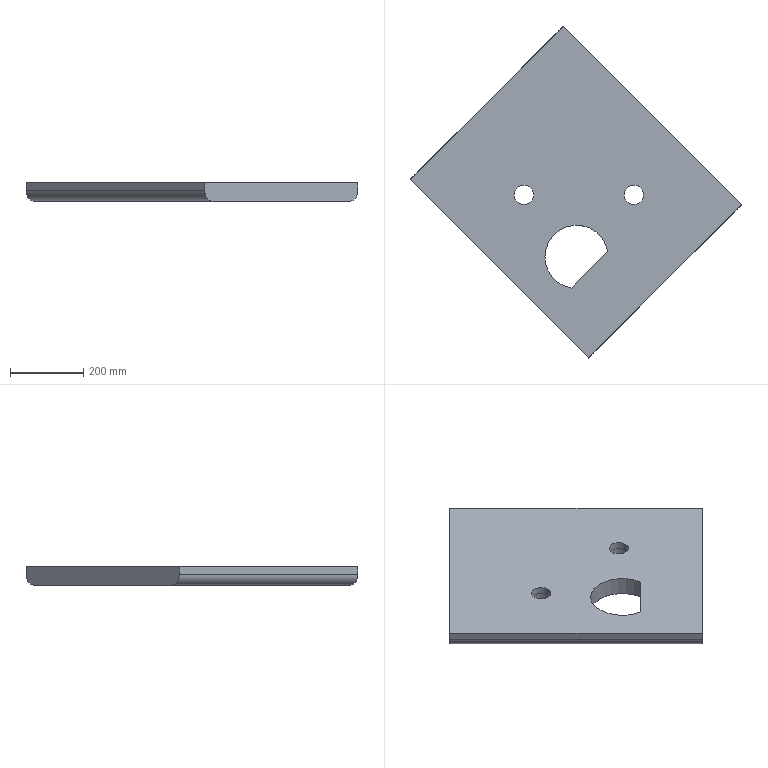Part | SolidWorks | 1 solid | 21 faces | box 906.604 x 906.604 x 50 mm | volume 18863747 mm3 | cylinder 12 | plane 9 | commonest cylinder face diameters 53 x4 68 x4 60 x2 172.729 x2
STEP:
#1=CARTESIAN_POINT('',(228.878,-154.889,-802.42));
#2=VERTEX_POINT('',#1);
#3=CARTESIAN_POINT('',(57.365,-169.327,-802.42));
#4=VERTEX_POINT('',#3);
#5=CARTESIAN_POINT('',(143.73,-169.327,-802.42));
#6=DIRECTION('',(0.,0.,1.));
#7=DIRECTION('',(0.9859,0.1672,0.));
#8=AXIS2_PLACEMENT_3D('',#5,#6,#7);
#9=CIRCLE('',#8,86.364);
#10=EDGE_CURVE('',#2,#4,#9,.T.);
#11=ORIENTED_EDGE('',*,*,#10,.T.);
#12=CARTESIAN_POINT('',(57.365,-169.327,-852.42));
#13=VERTEX_POINT('',#12);
#14=CARTESIAN_POINT('',(57.365,-169.327,-852.42));
#15=DIRECTION('',(0.,0.,-1.));
#16=VECTOR('',#15,1000.);
#17=LINE('',#14,#16);
#18=EDGE_CURVE('',#4,#13,#17,.T.);
#19=ORIENTED_EDGE('',*,*,#18,.T.);
#20=CARTESIAN_POINT('',(228.878,-154.889,-852.42));
#21=VERTEX_POINT('',#20);
#22=CARTESIAN_POINT('',(143.73,-169.327,-852.42));
#23=DIRECTION('',(0.,0.,-1.));
#24=DIRECTION('',(-0.1672,-0.9859,0.));
#25=AXIS2_PLACEMENT_3D('',#22,#23,#24);
#26=CIRCLE('',#25,86.364);
#27=EDGE_CURVE('',#13,#21,#26,.T.);
#28=ORIENTED_EDGE('',*,*,#27,.T.);
#29=CARTESIAN_POINT('',(228.878,-154.889,-802.42));
#30=DIRECTION('',(0.,0.,-1.));
#31=VECTOR('',#30,1000.);
#32=LINE('',#29,#31);
#33=EDGE_CURVE('',#2,#21,#32,.T.);
#34=ORIENTED_EDGE('',*,*,#33,.F.);
#35=EDGE_LOOP('',(#11,#19,#28,#34));
#36=FACE_OUTER_BOUND('',#35,.T.);
#37=CARTESIAN_POINT('',(143.73,-169.327,-852.42));
#38=DIRECTION('',(0.,0.,-1.));
#39=DIRECTION('',(-1.,0.,0.));
#40=AXIS2_PLACEMENT_3D('',#37,#38,#39);
#41=CYLINDRICAL_SURFACE('',#40,86.364);
#42=ADVANCED_FACE('',(#36),#41,.F.);
#43=ORIENTED_EDGE('',*,*,#18,.F.);
#44=CARTESIAN_POINT('',(129.291,-254.476,-802.42));
#45=VERTEX_POINT('',#44);
#46=CARTESIAN_POINT('',(143.73,-169.327,-802.42));
#47=DIRECTION('',(0.,0.,1.));
#48=DIRECTION('',(0.9859,0.1672,0.));
#49=AXIS2_PLACEMENT_3D('',#46,#47,#48);
#50=CIRCLE('',#49,86.364);
#51=EDGE_CURVE('',#4,#45,#50,.T.);
#52=ORIENTED_EDGE('',*,*,#51,.T.);
#53=CARTESIAN_POINT('',(129.291,-254.476,-852.42));
#54=VERTEX_POINT('',#53);
#55=CARTESIAN_POINT('',(129.291,-254.476,-852.42));
#56=DIRECTION('',(0.,0.,1.));
#57=VECTOR('',#56,1000.);
#58=LINE('',#55,#57);
#59=EDGE_CURVE('',#54,#45,#58,.T.);
#60=ORIENTED_EDGE('',*,*,#59,.F.);
#61=CARTESIAN_POINT('',(143.73,-169.327,-852.42));
#62=DIRECTION('',(0.,0.,-1.));
#63=DIRECTION('',(-0.1672,-0.9859,0.));
#64=AXIS2_PLACEMENT_3D('',#61,#62,#63);
#65=CIRCLE('',#64,86.364);
#66=EDGE_CURVE('',#54,#13,#65,.T.);
#67=ORIENTED_EDGE('',*,*,#66,.T.);
#68=EDGE_LOOP('',(#43,#52,#60,#67));
#69=FACE_OUTER_BOUND('',#68,.T.);
#70=CARTESIAN_POINT('',(143.73,-169.327,-852.42));
#71=DIRECTION('',(0.,0.,-1.));
#72=DIRECTION('',(-1.,0.,0.));
#73=AXIS2_PLACEMENT_3D('',#70,#71,#72);
#74=CYLINDRICAL_SURFACE('',#73,86.364);
#75=ADVANCED_FACE('',(#69),#74,.F.);
#76=CARTESIAN_POINT('',(129.291,-254.476,-802.42));
#77=DIRECTION('',(0.7071,0.7071,0.));
#78=VECTOR('',#77,1000.);
#79=LINE('',#76,#78);
#80=EDGE_CURVE('',#45,#2,#79,.T.);
#81=ORIENTED_EDGE('',*,*,#80,.T.);
#82=ORIENTED_EDGE('',*,*,#33,.T.);
#83=CARTESIAN_POINT('',(228.878,-154.889,-852.42));
#84=DIRECTION('',(-0.7071,-0.7071,0.));
#85=VECTOR('',#84,1000.);
#86=LINE('',#83,#85);
#87=EDGE_CURVE('',#21,#54,#86,.T.);
#88=ORIENTED_EDGE('',*,*,#87,.T.);
#89=ORIENTED_EDGE('',*,*,#59,.T.);
#90=EDGE_LOOP('',(#81,#82,#88,#89));
#91=FACE_OUTER_BOUND('',#90,.T.);
#92=CARTESIAN_POINT('',(240.322,-143.445,-852.42));
#93=DIRECTION('',(0.7071,-0.7071,0.));
#94=DIRECTION('',(0.,0.,-1.));
#95=AXIS2_PLACEMENT_3D('',#92,#93,#94);
#96=PLANE('',#95);
#97=ADVANCED_FACE('',(#91),#96,.F.);
#98=CARTESIAN_POINT('',(334.,0.,-822.42));
#99=VERTEX_POINT('',#98);
#100=CARTESIAN_POINT('',(266.,0.,-822.42));
#101=VERTEX_POINT('',#100);
#102=CARTESIAN_POINT('',(300.,0.,-822.42));
#103=DIRECTION('',(0.,0.,1.));
#104=DIRECTION('',(1.,0.,0.));
#105=AXIS2_PLACEMENT_3D('',#102,#103,#104);
#106=CIRCLE('',#105,34.);
#107=EDGE_CURVE('',#99,#101,#106,.T.);
#108=ORIENTED_EDGE('',*,*,#107,.T.);
#109=CARTESIAN_POINT('',(266.,0.,-852.42));
#110=VERTEX_POINT('',#109);
#111=CARTESIAN_POINT('',(266.,0.,-822.42));
#112=DIRECTION('',(0.,0.,-1.));
#113=VECTOR('',#112,1000.);
#114=LINE('',#111,#113);
#115=EDGE_CURVE('',#101,#110,#114,.T.);
#116=ORIENTED_EDGE('',*,*,#115,.T.);
#117=CARTESIAN_POINT('',(334.,0.,-852.42));
#118=VERTEX_POINT('',#117);
#119=CARTESIAN_POINT('',(300.,0.,-852.42));
#120=DIRECTION('',(0.,0.,-1.));
#121=DIRECTION('',(-1.,0.,0.));
#122=AXIS2_PLACEMENT_3D('',#119,#120,#121);
#123=CIRCLE('',#122,34.);
#124=EDGE_CURVE('',#110,#118,#123,.T.);
#125=ORIENTED_EDGE('',*,*,#124,.T.);
#126=CARTESIAN_POINT('',(334.,0.,-822.42));
#127=DIRECTION('',(0.,0.,-1.));
#128=VECTOR('',#127,1000.);
#129=LINE('',#126,#128);
#130=EDGE_CURVE('',#99,#118,#129,.T.);
#131=ORIENTED_EDGE('',*,*,#130,.F.);
#132=EDGE_LOOP('',(#108,#116,#125,#131));
#133=FACE_OUTER_BOUND('',#132,.T.);
#134=CARTESIAN_POINT('',(300.,0.,-852.42));
#135=DIRECTION('',(0.,0.,-1.));
#136=DIRECTION('',(-1.,0.,0.));
#137=AXIS2_PLACEMENT_3D('',#134,#135,#136);
#138=CYLINDRICAL_SURFACE('',#137,34.);
#139=ADVANCED_FACE('',(#133),#138,.F.);
#140=CARTESIAN_POINT('',(300.,0.,-822.42));
#141=DIRECTION('',(0.,0.,1.));
#142=DIRECTION('',(-1.,0.,0.));
#143=AXIS2_PLACEMENT_3D('',#140,#141,#142);
#144=CIRCLE('',#143,34.);
#145=EDGE_CURVE('',#101,#99,#144,.T.);
#146=ORIENTED_EDGE('',*,*,#145,.T.);
#147=ORIENTED_EDGE('',*,*,#130,.T.);
#148=CARTESIAN_POINT('',(300.,0.,-852.42));
#149=DIRECTION('',(0.,0.,-1.));
#150=DIRECTION('',(1.,0.,0.));
#151=AXIS2_PLACEMENT_3D('',#148,#149,#150);
#152=CIRCLE('',#151,34.);
#153=EDGE_CURVE('',#118,#110,#152,.T.);
#154=ORIENTED_EDGE('',*,*,#153,.T.);
#155=ORIENTED_EDGE('',*,*,#115,.F.);
#156=EDGE_LOOP('',(#146,#147,#154,#155));
#157=FACE_OUTER_BOUND('',#156,.T.);
#158=CARTESIAN_POINT('',(300.,0.,-852.42));
#159=DIRECTION('',(0.,0.,-1.));
#160=DIRECTION('',(-1.,0.,0.));
#161=AXIS2_PLACEMENT_3D('',#158,#159,#160);
#162=CYLINDRICAL_SURFACE('',#161,34.);
#163=ADVANCED_FACE('',(#157),#162,.F.);
#164=CARTESIAN_POINT('',(273.5,0.,-822.42));
#165=VERTEX_POINT('',#164);
#166=CARTESIAN_POINT('',(326.5,0.,-822.42));
#167=VERTEX_POINT('',#166);
#168=CARTESIAN_POINT('',(300.,0.,-822.42));
#169=DIRECTION('',(0.,0.,-1.));
#170=DIRECTION('',(-1.,0.,0.));
#171=AXIS2_PLACEMENT_3D('',#168,#169,#170);
#172=CIRCLE('',#171,26.5);
#173=EDGE_CURVE('',#165,#167,#172,.T.);
#174=ORIENTED_EDGE('',*,*,#173,.F.);
#175=CARTESIAN_POINT('',(300.,0.,-822.42));
#176=DIRECTION('',(0.,0.,-1.));
#177=DIRECTION('',(1.,0.,0.));
#178=AXIS2_PLACEMENT_3D('',#175,#176,#177);
#179=CIRCLE('',#178,26.5);
#180=EDGE_CURVE('',#167,#165,#179,.T.);
#181=ORIENTED_EDGE('',*,*,#180,.F.);
#182=EDGE_LOOP('',(#174,#181));
#183=FACE_BOUND('',#182,.T.);
#184=ORIENTED_EDGE('',*,*,#107,.F.);
#185=ORIENTED_EDGE('',*,*,#145,.F.);
#186=EDGE_LOOP('',(#184,#185));
#187=FACE_OUTER_BOUND('',#186,.T.);
#188=CARTESIAN_POINT('',(0.,0.,-822.42));
#189=DIRECTION('',(0.,0.,-1.));
#190=DIRECTION('',(0.,-1.,0.));
#191=AXIS2_PLACEMENT_3D('',#188,#189,#190);
#192=PLANE('',#191);
#193=ADVANCED_FACE('',(#183,#187),#192,.T.);
#194=CARTESIAN_POINT('',(326.5,0.,-802.42));
#195=VERTEX_POINT('',#194);
#196=CARTESIAN_POINT('',(273.5,0.,-802.42));
#197=VERTEX_POINT('',#196);
#198=CARTESIAN_POINT('',(300.,0.,-802.42));
#199=DIRECTION('',(0.,0.,1.));
#200=DIRECTION('',(1.,0.,0.));
#201=AXIS2_PLACEMENT_3D('',#198,#199,#200);
#202=CIRCLE('',#201,26.5);
#203=EDGE_CURVE('',#195,#197,#202,.T.);
#204=ORIENTED_EDGE('',*,*,#203,.T.);
#205=CARTESIAN_POINT('',(273.5,0.,-802.42));
#206=DIRECTION('',(0.,0.,-1.));
#207=VECTOR('',#206,1000.);
#208=LINE('',#205,#207);
#209=EDGE_CURVE('',#197,#165,#208,.T.);
#210=ORIENTED_EDGE('',*,*,#209,.T.);
#211=ORIENTED_EDGE('',*,*,#173,.T.);
#212=CARTESIAN_POINT('',(326.5,0.,-802.42));
#213=DIRECTION('',(0.,0.,-1.));
#214=VECTOR('',#213,1000.);
#215=LINE('',#212,#214);
#216=EDGE_CURVE('',#195,#167,#215,.T.);
#217=ORIENTED_EDGE('',*,*,#216,.F.);
#218=EDGE_LOOP('',(#204,#210,#211,#217));
#219=FACE_OUTER_BOUND('',#218,.T.);
#220=CARTESIAN_POINT('',(300.,0.,-852.42));
#221=DIRECTION('',(0.,0.,-1.));
#222=DIRECTION('',(-1.,0.,0.));
#223=AXIS2_PLACEMENT_3D('',#220,#221,#222);
#224=CYLINDRICAL_SURFACE('',#223,26.5);
#225=ADVANCED_FACE('',(#219),#224,.F.);
#226=CARTESIAN_POINT('',(300.,0.,-802.42));
#227=DIRECTION('',(0.,0.,1.));
#228=DIRECTION('',(-1.,0.,0.));
#229=AXIS2_PLACEMENT_3D('',#226,#227,#228);
#230=CIRCLE('',#229,26.5);
#231=EDGE_CURVE('',#197,#195,#230,.T.);
#232=ORIENTED_EDGE('',*,*,#231,.T.);
#233=ORIENTED_EDGE('',*,*,#216,.T.);
#234=ORIENTED_EDGE('',*,*,#180,.T.);
#235=ORIENTED_EDGE('',*,*,#209,.F.);
#236=EDGE_LOOP('',(#232,#233,#234,#235));
#237=FACE_OUTER_BOUND('',#236,.T.);
#238=CARTESIAN_POINT('',(300.,0.,-852.42));
#239=DIRECTION('',(0.,0.,-1.));
#240=DIRECTION('',(-1.,0.,0.));
#241=AXIS2_PLACEMENT_3D('',#238,#239,#240);
#242=CYLINDRICAL_SURFACE('',#241,26.5);
#243=ADVANCED_FACE('',(#237),#242,.F.);
#244=ORIENTED_EDGE('',*,*,#80,.F.);
#245=ORIENTED_EDGE('',*,*,#51,.F.);
#246=ORIENTED_EDGE('',*,*,#10,.F.);
#247=EDGE_LOOP('',(#244,#245,#246));
#248=FACE_BOUND('',#247,.T.);
#249=CARTESIAN_POINT('',(26.5,0.,-802.42));
#250=VERTEX_POINT('',#249);
#251=CARTESIAN_POINT('',(-26.5,0.,-802.42));
#252=VERTEX_POINT('',#251);
#253=CARTESIAN_POINT('',(0.,0.,-802.42));
#254=DIRECTION('',(0.,0.,1.));
#255=DIRECTION('',(1.,0.,0.));
#256=AXIS2_PLACEMENT_3D('',#253,#254,#255);
#257=CIRCLE('',#256,26.5);
#258=EDGE_CURVE('',#250,#252,#257,.T.);
#259=ORIENTED_EDGE('',*,*,#258,.F.);
#260=CARTESIAN_POINT('',(0.,0.,-802.42));
#261=DIRECTION('',(0.,0.,1.));
#262=DIRECTION('',(-1.,0.,0.));
#263=AXIS2_PLACEMENT_3D('',#260,#261,#262);
#264=CIRCLE('',#263,26.5);
#265=EDGE_CURVE('',#252,#250,#264,.T.);
#266=ORIENTED_EDGE('',*,*,#265,.F.);
#267=EDGE_LOOP('',(#259,#266));
#268=FACE_BOUND('',#267,.T.);
#269=ORIENTED_EDGE('',*,*,#203,.F.);
#270=ORIENTED_EDGE('',*,*,#231,.F.);
#271=EDGE_LOOP('',(#269,#270));
#272=FACE_BOUND('',#271,.T.);
#273=CARTESIAN_POINT('',(-311.127,42.426,-802.42));
#274=VERTEX_POINT('',#273);
#275=CARTESIAN_POINT('',(107.574,461.127,-802.42));
#276=VERTEX_POINT('',#275);
#277=CARTESIAN_POINT('',(-311.127,42.426,-802.42));
#278=DIRECTION('',(0.7071,0.7071,0.));
#279=VECTOR('',#278,1000.);
#280=LINE('',#277,#279);
#281=EDGE_CURVE('',#274,#276,#280,.T.);
#282=ORIENTED_EDGE('',*,*,#281,.F.);
#283=CARTESIAN_POINT('',(176.777,-445.477,-802.42));
#284=VERTEX_POINT('',#283);
#285=CARTESIAN_POINT('',(176.777,-445.477,-802.42));
#286=DIRECTION('',(-0.7071,0.7071,0.));
#287=VECTOR('',#286,1000.);
#288=LINE('',#285,#287);
#289=EDGE_CURVE('',#284,#274,#288,.T.);
#290=ORIENTED_EDGE('',*,*,#289,.F.);
#291=CARTESIAN_POINT('',(595.477,-26.777,-802.42));
#292=VERTEX_POINT('',#291);
#293=CARTESIAN_POINT('',(595.477,-26.777,-802.42));
#294=DIRECTION('',(-0.7071,-0.7071,0.));
#295=VECTOR('',#294,1000.);
#296=LINE('',#293,#295);
#297=EDGE_CURVE('',#292,#284,#296,.T.);
#298=ORIENTED_EDGE('',*,*,#297,.F.);
#299=CARTESIAN_POINT('',(107.574,461.127,-802.42));
#300=DIRECTION('',(0.7071,-0.7071,0.));
#301=VECTOR('',#300,1000.);
#302=LINE('',#299,#301);
#303=EDGE_CURVE('',#276,#292,#302,.T.);
#304=ORIENTED_EDGE('',*,*,#303,.F.);
#305=EDGE_LOOP('',(#282,#290,#298,#304));
#306=FACE_OUTER_BOUND('',#305,.T.);
#307=CARTESIAN_POINT('',(0.,0.,-802.42));
#308=DIRECTION('',(0.,0.,-1.));
#309=DIRECTION('',(0.,-1.,0.));
#310=AXIS2_PLACEMENT_3D('',#307,#308,#309);
#311=PLANE('',#310);
#312=ADVANCED_FACE('',(#248,#268,#272,#306),#311,.F.);
#313=CARTESIAN_POINT('',(197.99,-424.264,-852.42));
#314=VERTEX_POINT('',#313);
#315=CARTESIAN_POINT('',(574.264,-47.99,-852.42));
#316=VERTEX_POINT('',#315);
#317=CARTESIAN_POINT('',(176.777,-445.477,-852.42));
#318=DIRECTION('',(0.7071,0.7071,0.));
#319=VECTOR('',#318,1000.);
#320=LINE('',#317,#319);
#321=EDGE_CURVE('',#314,#316,#320,.T.);
#322=ORIENTED_EDGE('',*,*,#321,.T.);
#323=CARTESIAN_POINT('',(595.477,-26.777,-822.42));
#324=VERTEX_POINT('',#323);
#325=CARTESIAN_POINT('',(574.264,-47.99,-822.42));
#326=DIRECTION('',(0.7071,-0.7071,0.));
#327=DIRECTION('',(0.7071,0.7071,0.));
#328=AXIS2_PLACEMENT_3D('',#325,#326,#327);
#329=CIRCLE('',#328,30.);
#330=EDGE_CURVE('',#316,#324,#329,.T.);
#331=ORIENTED_EDGE('',*,*,#330,.T.);
#332=CARTESIAN_POINT('',(595.477,-26.777,-852.42));
#333=DIRECTION('',(0.,0.,1.));
#334=VECTOR('',#333,1000.);
#335=LINE('',#332,#334);
#336=EDGE_CURVE('',#324,#292,#335,.T.);
#337=ORIENTED_EDGE('',*,*,#336,.T.);
#338=ORIENTED_EDGE('',*,*,#297,.T.);
#339=CARTESIAN_POINT('',(176.777,-445.477,-822.42));
#340=VERTEX_POINT('',#339);
#341=CARTESIAN_POINT('',(176.777,-445.477,-852.42));
#342=DIRECTION('',(0.,0.,1.));
#343=VECTOR('',#342,1000.);
#344=LINE('',#341,#343);
#345=EDGE_CURVE('',#340,#284,#344,.T.);
#346=ORIENTED_EDGE('',*,*,#345,.F.);
#347=CARTESIAN_POINT('',(197.99,-424.264,-822.42));
#348=DIRECTION('',(0.7071,-0.7071,0.));
#349=DIRECTION('',(0.7071,0.7071,0.));
#350=AXIS2_PLACEMENT_3D('',#347,#348,#349);
#351=CIRCLE('',#350,30.);
#352=EDGE_CURVE('',#340,#314,#351,.T.);
#353=ORIENTED_EDGE('',*,*,#352,.T.);
#354=EDGE_LOOP('',(#322,#331,#337,#338,#346,#353));
#355=FACE_OUTER_BOUND('',#354,.T.);
#356=CARTESIAN_POINT('',(595.477,-26.777,-802.42));
#357=DIRECTION('',(0.7071,-0.7071,0.));
#358=DIRECTION('',(0.,0.,-1.));
#359=AXIS2_PLACEMENT_3D('',#356,#357,#358);
#360=PLANE('',#359);
#361=ADVANCED_FACE('',(#355),#360,.T.);
#362=ORIENTED_EDGE('',*,*,#336,.F.);
#363=CARTESIAN_POINT('',(107.574,461.127,-822.42));
#364=VERTEX_POINT('',#363);
#365=CARTESIAN_POINT('',(107.574,461.127,-822.42));
#366=DIRECTION('',(-0.7071,0.7071,0.));
#367=VECTOR('',#366,1000.);
#368=LINE('',#365,#367);
#369=EDGE_CURVE('',#324,#364,#368,.T.);
#370=ORIENTED_EDGE('',*,*,#369,.T.);
#371=CARTESIAN_POINT('',(107.574,461.127,-852.42));
#372=DIRECTION('',(0.,0.,1.));
#373=VECTOR('',#372,1000.);
#374=LINE('',#371,#373);
#375=EDGE_CURVE('',#364,#276,#374,.T.);
#376=ORIENTED_EDGE('',*,*,#375,.T.);
#377=ORIENTED_EDGE('',*,*,#303,.T.);
#378=EDGE_LOOP('',(#362,#370,#376,#377));
#379=FACE_OUTER_BOUND('',#378,.T.);
#380=CARTESIAN_POINT('',(107.574,461.127,-802.42));
#381=DIRECTION('',(0.7071,0.7071,0.));
#382=DIRECTION('',(0.,0.,-1.));
#383=AXIS2_PLACEMENT_3D('',#380,#381,#382);
#384=PLANE('',#383);
#385=ADVANCED_FACE('',(#379),#384,.T.);
#386=ORIENTED_EDGE('',*,*,#375,.F.);
#387=CARTESIAN_POINT('',(86.36,439.914,-852.42));
#388=VERTEX_POINT('',#387);
#389=CARTESIAN_POINT('',(86.36,439.914,-822.42));
#390=DIRECTION('',(-0.7071,0.7071,0.));
#391=DIRECTION('',(-0.7071,-0.7071,0.));
#392=AXIS2_PLACEMENT_3D('',#389,#390,#391);
#393=CIRCLE('',#392,30.);
#394=EDGE_CURVE('',#364,#388,#393,.T.);
#395=ORIENTED_EDGE('',*,*,#394,.T.);
#396=CARTESIAN_POINT('',(-289.914,63.64,-852.42));
#397=VERTEX_POINT('',#396);
#398=CARTESIAN_POINT('',(107.574,461.127,-852.42));
#399=DIRECTION('',(-0.7071,-0.7071,0.));
#400=VECTOR('',#399,1000.);
#401=LINE('',#398,#400);
#402=EDGE_CURVE('',#388,#397,#401,.T.);
#403=ORIENTED_EDGE('',*,*,#402,.T.);
#404=CARTESIAN_POINT('',(-311.127,42.426,-822.42));
#405=VERTEX_POINT('',#404);
#406=CARTESIAN_POINT('',(-289.914,63.64,-822.42));
#407=DIRECTION('',(-0.7071,0.7071,0.));
#408=DIRECTION('',(-0.7071,-0.7071,0.));
#409=AXIS2_PLACEMENT_3D('',#406,#407,#408);
#410=CIRCLE('',#409,30.);
#411=EDGE_CURVE('',#397,#405,#410,.T.);
#412=ORIENTED_EDGE('',*,*,#411,.T.);
#413=CARTESIAN_POINT('',(-311.127,42.426,-852.42));
#414=DIRECTION('',(0.,0.,1.));
#415=VECTOR('',#414,1000.);
#416=LINE('',#413,#415);
#417=EDGE_CURVE('',#405,#274,#416,.T.);
#418=ORIENTED_EDGE('',*,*,#417,.T.);
#419=ORIENTED_EDGE('',*,*,#281,.T.);
#420=EDGE_LOOP('',(#386,#395,#403,#412,#418,#419));
#421=FACE_OUTER_BOUND('',#420,.T.);
#422=CARTESIAN_POINT('',(-311.127,42.426,-802.42));
#423=DIRECTION('',(-0.7071,0.7071,0.));
#424=DIRECTION('',(0.,0.,1.));
#425=AXIS2_PLACEMENT_3D('',#422,#423,#424);
#426=PLANE('',#425);
#427=ADVANCED_FACE('',(#421),#426,.T.);
#428=ORIENTED_EDGE('',*,*,#417,.F.);
#429=CARTESIAN_POINT('',(176.777,-445.477,-822.42));
#430=DIRECTION('',(0.7071,-0.7071,0.));
#431=VECTOR('',#430,1000.);
#432=LINE('',#429,#431);
#433=EDGE_CURVE('',#405,#340,#432,.T.);
#434=ORIENTED_EDGE('',*,*,#433,.T.);
#435=ORIENTED_EDGE('',*,*,#345,.T.);
#436=ORIENTED_EDGE('',*,*,#289,.T.);
#437=EDGE_LOOP('',(#428,#434,#435,#436));
#438=FACE_OUTER_BOUND('',#437,.T.);
#439=CARTESIAN_POINT('',(176.777,-445.477,-802.42));
#440=DIRECTION('',(-0.7071,-0.7071,0.));
#441=DIRECTION('',(-0.7071,0.7071,0.));
#442=AXIS2_PLACEMENT_3D('',#439,#440,#441);
#443=PLANE('',#442);
#444=ADVANCED_FACE('',(#438),#443,.T.);
#445=ORIENTED_EDGE('',*,*,#87,.F.);
#446=ORIENTED_EDGE('',*,*,#27,.F.);
#447=ORIENTED_EDGE('',*,*,#66,.F.);
#448=EDGE_LOOP('',(#445,#446,#447));
#449=FACE_BOUND('',#448,.T.);
#450=CARTESIAN_POINT('',(-34.,0.,-852.42));
#451=VERTEX_POINT('',#450);
#452=CARTESIAN_POINT('',(34.,0.,-852.42));
#453=VERTEX_POINT('',#452);
#454=CARTESIAN_POINT('',(0.,0.,-852.42));
#455=DIRECTION('',(0.,0.,-1.));
#456=DIRECTION('',(-1.,0.,0.));
#457=AXIS2_PLACEMENT_3D('',#454,#455,#456);
#458=CIRCLE('',#457,34.);
#459=EDGE_CURVE('',#451,#453,#458,.T.);
#460=ORIENTED_EDGE('',*,*,#459,.F.);
#461=CARTESIAN_POINT('',(0.,0.,-852.42));
#462=DIRECTION('',(0.,0.,-1.));
#463=DIRECTION('',(1.,0.,0.));
#464=AXIS2_PLACEMENT_3D('',#461,#462,#463);
#465=CIRCLE('',#464,34.);
#466=EDGE_CURVE('',#453,#451,#465,.T.);
#467=ORIENTED_EDGE('',*,*,#466,.F.);
#468=EDGE_LOOP('',(#460,#467));
#469=FACE_BOUND('',#468,.T.);
#470=ORIENTED_EDGE('',*,*,#124,.F.);
#471=ORIENTED_EDGE('',*,*,#153,.F.);
#472=EDGE_LOOP('',(#470,#471));
#473=FACE_BOUND('',#472,.T.);
#474=ORIENTED_EDGE('',*,*,#402,.F.);
#475=CARTESIAN_POINT('',(263.137,263.137,-852.42));
#476=DIRECTION('',(0.7071,-0.7071,0.));
#477=VECTOR('',#476,1000.);
#478=LINE('',#475,#477);
#479=EDGE_CURVE('',#388,#316,#478,.T.);
#480=ORIENTED_EDGE('',*,*,#479,.T.);
#481=ORIENTED_EDGE('',*,*,#321,.F.);
#482=CARTESIAN_POINT('',(-113.137,-113.137,-852.42));
#483=DIRECTION('',(-0.7071,0.7071,0.));
#484=VECTOR('',#483,1000.);
#485=LINE('',#482,#484);
#486=EDGE_CURVE('',#314,#397,#485,.T.);
#487=ORIENTED_EDGE('',*,*,#486,.T.);
#488=EDGE_LOOP('',(#474,#480,#481,#487));
#489=FACE_OUTER_BOUND('',#488,.T.);
#490=CARTESIAN_POINT('',(0.,0.,-852.42));
#491=DIRECTION('',(0.,0.,-1.));
#492=DIRECTION('',(0.,-1.,0.));
#493=AXIS2_PLACEMENT_3D('',#490,#491,#492);
#494=PLANE('',#493);
#495=ADVANCED_FACE('',(#449,#469,#473,#489),#494,.T.);
#496=CARTESIAN_POINT('',(34.,0.,-822.42));
#497=VERTEX_POINT('',#496);
#498=CARTESIAN_POINT('',(-34.,0.,-822.42));
#499=VERTEX_POINT('',#498);
#500=CARTESIAN_POINT('',(0.,0.,-822.42));
#501=DIRECTION('',(0.,0.,1.));
#502=DIRECTION('',(1.,0.,0.));
#503=AXIS2_PLACEMENT_3D('',#500,#501,#502);
#504=CIRCLE('',#503,34.);
#505=EDGE_CURVE('',#497,#499,#504,.T.);
#506=ORIENTED_EDGE('',*,*,#505,.T.);
#507=CARTESIAN_POINT('',(-34.,0.,-822.42));
#508=DIRECTION('',(0.,0.,-1.));
#509=VECTOR('',#508,1000.);
#510=LINE('',#507,#509);
#511=EDGE_CURVE('',#499,#451,#510,.T.);
#512=ORIENTED_EDGE('',*,*,#511,.T.);
#513=ORIENTED_EDGE('',*,*,#459,.T.);
#514=CARTESIAN_POINT('',(34.,0.,-822.42));
#515=DIRECTION('',(0.,0.,-1.));
#516=VECTOR('',#515,1000.);
#517=LINE('',#514,#516);
#518=EDGE_CURVE('',#497,#453,#517,.T.);
#519=ORIENTED_EDGE('',*,*,#518,.F.);
#520=EDGE_LOOP('',(#506,#512,#513,#519));
#521=FACE_OUTER_BOUND('',#520,.T.);
#522=CARTESIAN_POINT('',(0.,0.,-852.42));
#523=DIRECTION('',(0.,0.,-1.));
#524=DIRECTION('',(-1.,0.,0.));
#525=AXIS2_PLACEMENT_3D('',#522,#523,#524);
#526=CYLINDRICAL_SURFACE('',#525,34.);
#527=ADVANCED_FACE('',(#521),#526,.F.);
#528=CARTESIAN_POINT('',(0.,0.,-822.42));
#529=DIRECTION('',(0.,0.,1.));
#530=DIRECTION('',(-1.,0.,0.));
#531=AXIS2_PLACEMENT_3D('',#528,#529,#530);
#532=CIRCLE('',#531,34.);
#533=EDGE_CURVE('',#499,#497,#532,.T.);
#534=ORIENTED_EDGE('',*,*,#533,.T.);
#535=ORIENTED_EDGE('',*,*,#518,.T.);
#536=ORIENTED_EDGE('',*,*,#466,.T.);
#537=ORIENTED_EDGE('',*,*,#511,.F.);
#538=EDGE_LOOP('',(#534,#535,#536,#537));
#539=FACE_OUTER_BOUND('',#538,.T.);
#540=CARTESIAN_POINT('',(0.,0.,-852.42));
#541=DIRECTION('',(0.,0.,-1.));
#542=DIRECTION('',(-1.,0.,0.));
#543=AXIS2_PLACEMENT_3D('',#540,#541,#542);
#544=CYLINDRICAL_SURFACE('',#543,34.);
#545=ADVANCED_FACE('',(#539),#544,.F.);
#546=CARTESIAN_POINT('',(-26.5,0.,-822.42));
#547=VERTEX_POINT('',#546);
#548=CARTESIAN_POINT('',(26.5,0.,-822.42));
#549=VERTEX_POINT('',#548);
#550=CARTESIAN_POINT('',(0.,0.,-822.42));
#551=DIRECTION('',(0.,0.,-1.));
#552=DIRECTION('',(-1.,0.,0.));
#553=AXIS2_PLACEMENT_3D('',#550,#551,#552);
#554=CIRCLE('',#553,26.5);
#555=EDGE_CURVE('',#547,#549,#554,.T.);
#556=ORIENTED_EDGE('',*,*,#555,.F.);
#557=CARTESIAN_POINT('',(0.,0.,-822.42));
#558=DIRECTION('',(0.,0.,-1.));
#559=DIRECTION('',(1.,0.,0.));
#560=AXIS2_PLACEMENT_3D('',#557,#558,#559);
#561=CIRCLE('',#560,26.5);
#562=EDGE_CURVE('',#549,#547,#561,.T.);
#563=ORIENTED_EDGE('',*,*,#562,.F.);
#564=EDGE_LOOP('',(#556,#563));
#565=FACE_BOUND('',#564,.T.);
#566=ORIENTED_EDGE('',*,*,#505,.F.);
#567=ORIENTED_EDGE('',*,*,#533,.F.);
#568=EDGE_LOOP('',(#566,#567));
#569=FACE_OUTER_BOUND('',#568,.T.);
#570=CARTESIAN_POINT('',(0.,0.,-822.42));
#571=DIRECTION('',(0.,0.,-1.));
#572=DIRECTION('',(0.,-1.,0.));
#573=AXIS2_PLACEMENT_3D('',#570,#571,#572);
#574=PLANE('',#573);
#575=ADVANCED_FACE('',(#565,#569),#574,.T.);
#576=ORIENTED_EDGE('',*,*,#265,.T.);
#577=CARTESIAN_POINT('',(26.5,0.,-802.42));
#578=DIRECTION('',(0.,0.,-1.));
#579=VECTOR('',#578,1000.);
#580=LINE('',#577,#579);
#581=EDGE_CURVE('',#250,#549,#580,.T.);
#582=ORIENTED_EDGE('',*,*,#581,.T.);
#583=ORIENTED_EDGE('',*,*,#562,.T.);
#584=CARTESIAN_POINT('',(-26.5,0.,-802.42));
#585=DIRECTION('',(0.,0.,-1.));
#586=VECTOR('',#585,1000.);
#587=LINE('',#584,#586);
#588=EDGE_CURVE('',#252,#547,#587,.T.);
#589=ORIENTED_EDGE('',*,*,#588,.F.);
#590=EDGE_LOOP('',(#576,#582,#583,#589));
#591=FACE_OUTER_BOUND('',#590,.T.);
#592=CARTESIAN_POINT('',(0.,0.,-852.42));
#593=DIRECTION('',(0.,0.,-1.));
#594=DIRECTION('',(-1.,0.,0.));
#595=AXIS2_PLACEMENT_3D('',#592,#593,#594);
#596=CYLINDRICAL_SURFACE('',#595,26.5);
#597=ADVANCED_FACE('',(#591),#596,.F.);
#598=ORIENTED_EDGE('',*,*,#258,.T.);
#599=ORIENTED_EDGE('',*,*,#588,.T.);
#600=ORIENTED_EDGE('',*,*,#555,.T.);
#601=ORIENTED_EDGE('',*,*,#581,.F.);
#602=EDGE_LOOP('',(#598,#599,#600,#601));
#603=FACE_OUTER_BOUND('',#602,.T.);
#604=CARTESIAN_POINT('',(0.,0.,-852.42));
#605=DIRECTION('',(0.,0.,-1.));
#606=DIRECTION('',(-1.,0.,0.));
#607=AXIS2_PLACEMENT_3D('',#604,#605,#606);
#608=CYLINDRICAL_SURFACE('',#607,26.5);
#609=ADVANCED_FACE('',(#603),#608,.F.);
#610=ORIENTED_EDGE('',*,*,#330,.F.);
#611=ORIENTED_EDGE('',*,*,#479,.F.);
#612=ORIENTED_EDGE('',*,*,#394,.F.);
#613=ORIENTED_EDGE('',*,*,#369,.F.);
#614=EDGE_LOOP('',(#610,#611,#612,#613));
#615=FACE_OUTER_BOUND('',#614,.T.);
#616=CARTESIAN_POINT('',(86.36,439.914,-822.42));
#617=DIRECTION('',(-0.7071,0.7071,0.));
#618=DIRECTION('',(-0.7071,-0.7071,0.));
#619=AXIS2_PLACEMENT_3D('',#616,#617,#618);
#620=CYLINDRICAL_SURFACE('',#619,30.);
#621=ADVANCED_FACE('',(#615),#620,.T.);
#622=ORIENTED_EDGE('',*,*,#411,.F.);
#623=ORIENTED_EDGE('',*,*,#486,.F.);
#624=ORIENTED_EDGE('',*,*,#352,.F.);
#625=ORIENTED_EDGE('',*,*,#433,.F.);
#626=EDGE_LOOP('',(#622,#623,#624,#625));
#627=FACE_OUTER_BOUND('',#626,.T.);
#628=CARTESIAN_POINT('',(197.99,-424.264,-822.42));
#629=DIRECTION('',(0.7071,-0.7071,0.));
#630=DIRECTION('',(0.7071,0.7071,0.));
#631=AXIS2_PLACEMENT_3D('',#628,#629,#630);
#632=CYLINDRICAL_SURFACE('',#631,30.);
#633=ADVANCED_FACE('',(#627),#632,.T.);
#634=CLOSED_SHELL('',(#42,#75,#97,#139,#163,#193,#225,#243,#312,#361,#385,#427,#444,#495,#527,#545,#575,#597,#609,#621,#633));
#635=MANIFOLD_SOLID_BREP('',#634);
#636=CARTESIAN_POINT('',(0.,0.,0.));
#637=DIRECTION('',(0.,0.,1.));
#638=DIRECTION('',(1.,0.,0.));
#639=AXIS2_PLACEMENT_3D('',#636,#637,#638);
#640=(LENGTH_UNIT()NAMED_UNIT(*)SI_UNIT(.MILLI.,.METRE.));
#641=UNCERTAINTY_MEASURE_WITH_UNIT(LENGTH_MEASURE(0.00001),#640,'','');
#642=(NAMED_UNIT(*)PLANE_ANGLE_UNIT()SI_UNIT($,.RADIAN.));
#643=(NAMED_UNIT(*)SI_UNIT($,.STERADIAN.)SOLID_ANGLE_UNIT());
#644=(GEOMETRIC_REPRESENTATION_CONTEXT(3)GLOBAL_UNCERTAINTY_ASSIGNED_CONTEXT((#641))GLOBAL_UNIT_ASSIGNED_CONTEXT((#640,#642,#643))REPRESENTATION_CONTEXT('',''));
#645=ADVANCED_BREP_SHAPE_REPRESENTATION('',(#635,#639),#644);